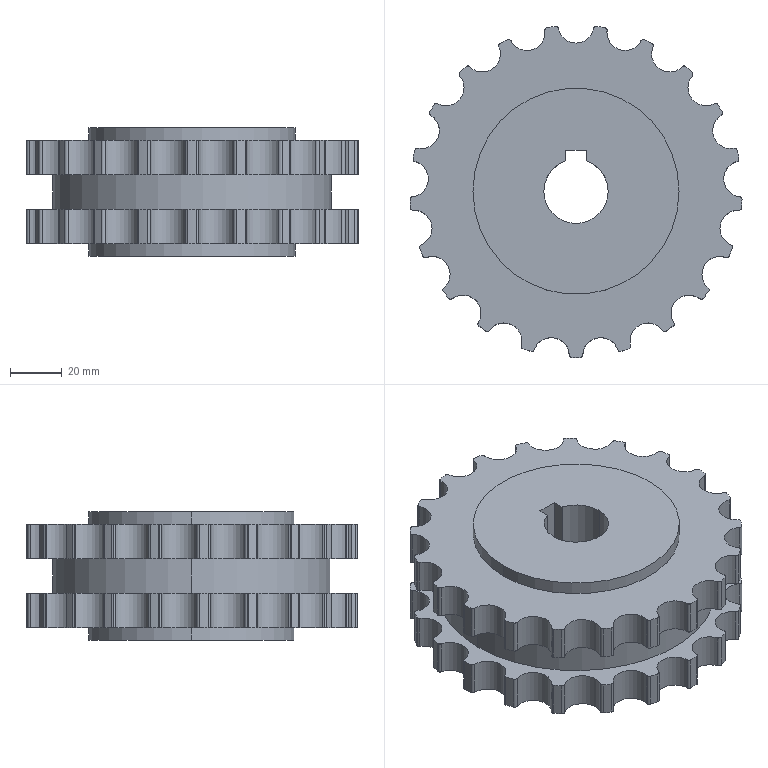Part | SolidWorks | features BaseBody 1 | 1 solid | 224 faces | box 128.846 x 128.512 x 50 mm | volume 452418 mm3 | cylinder 215 | plane 9 | commonest cylinder face diameters 2 x104 14 x60 129 x42 80 x4 25 x3 108 x2